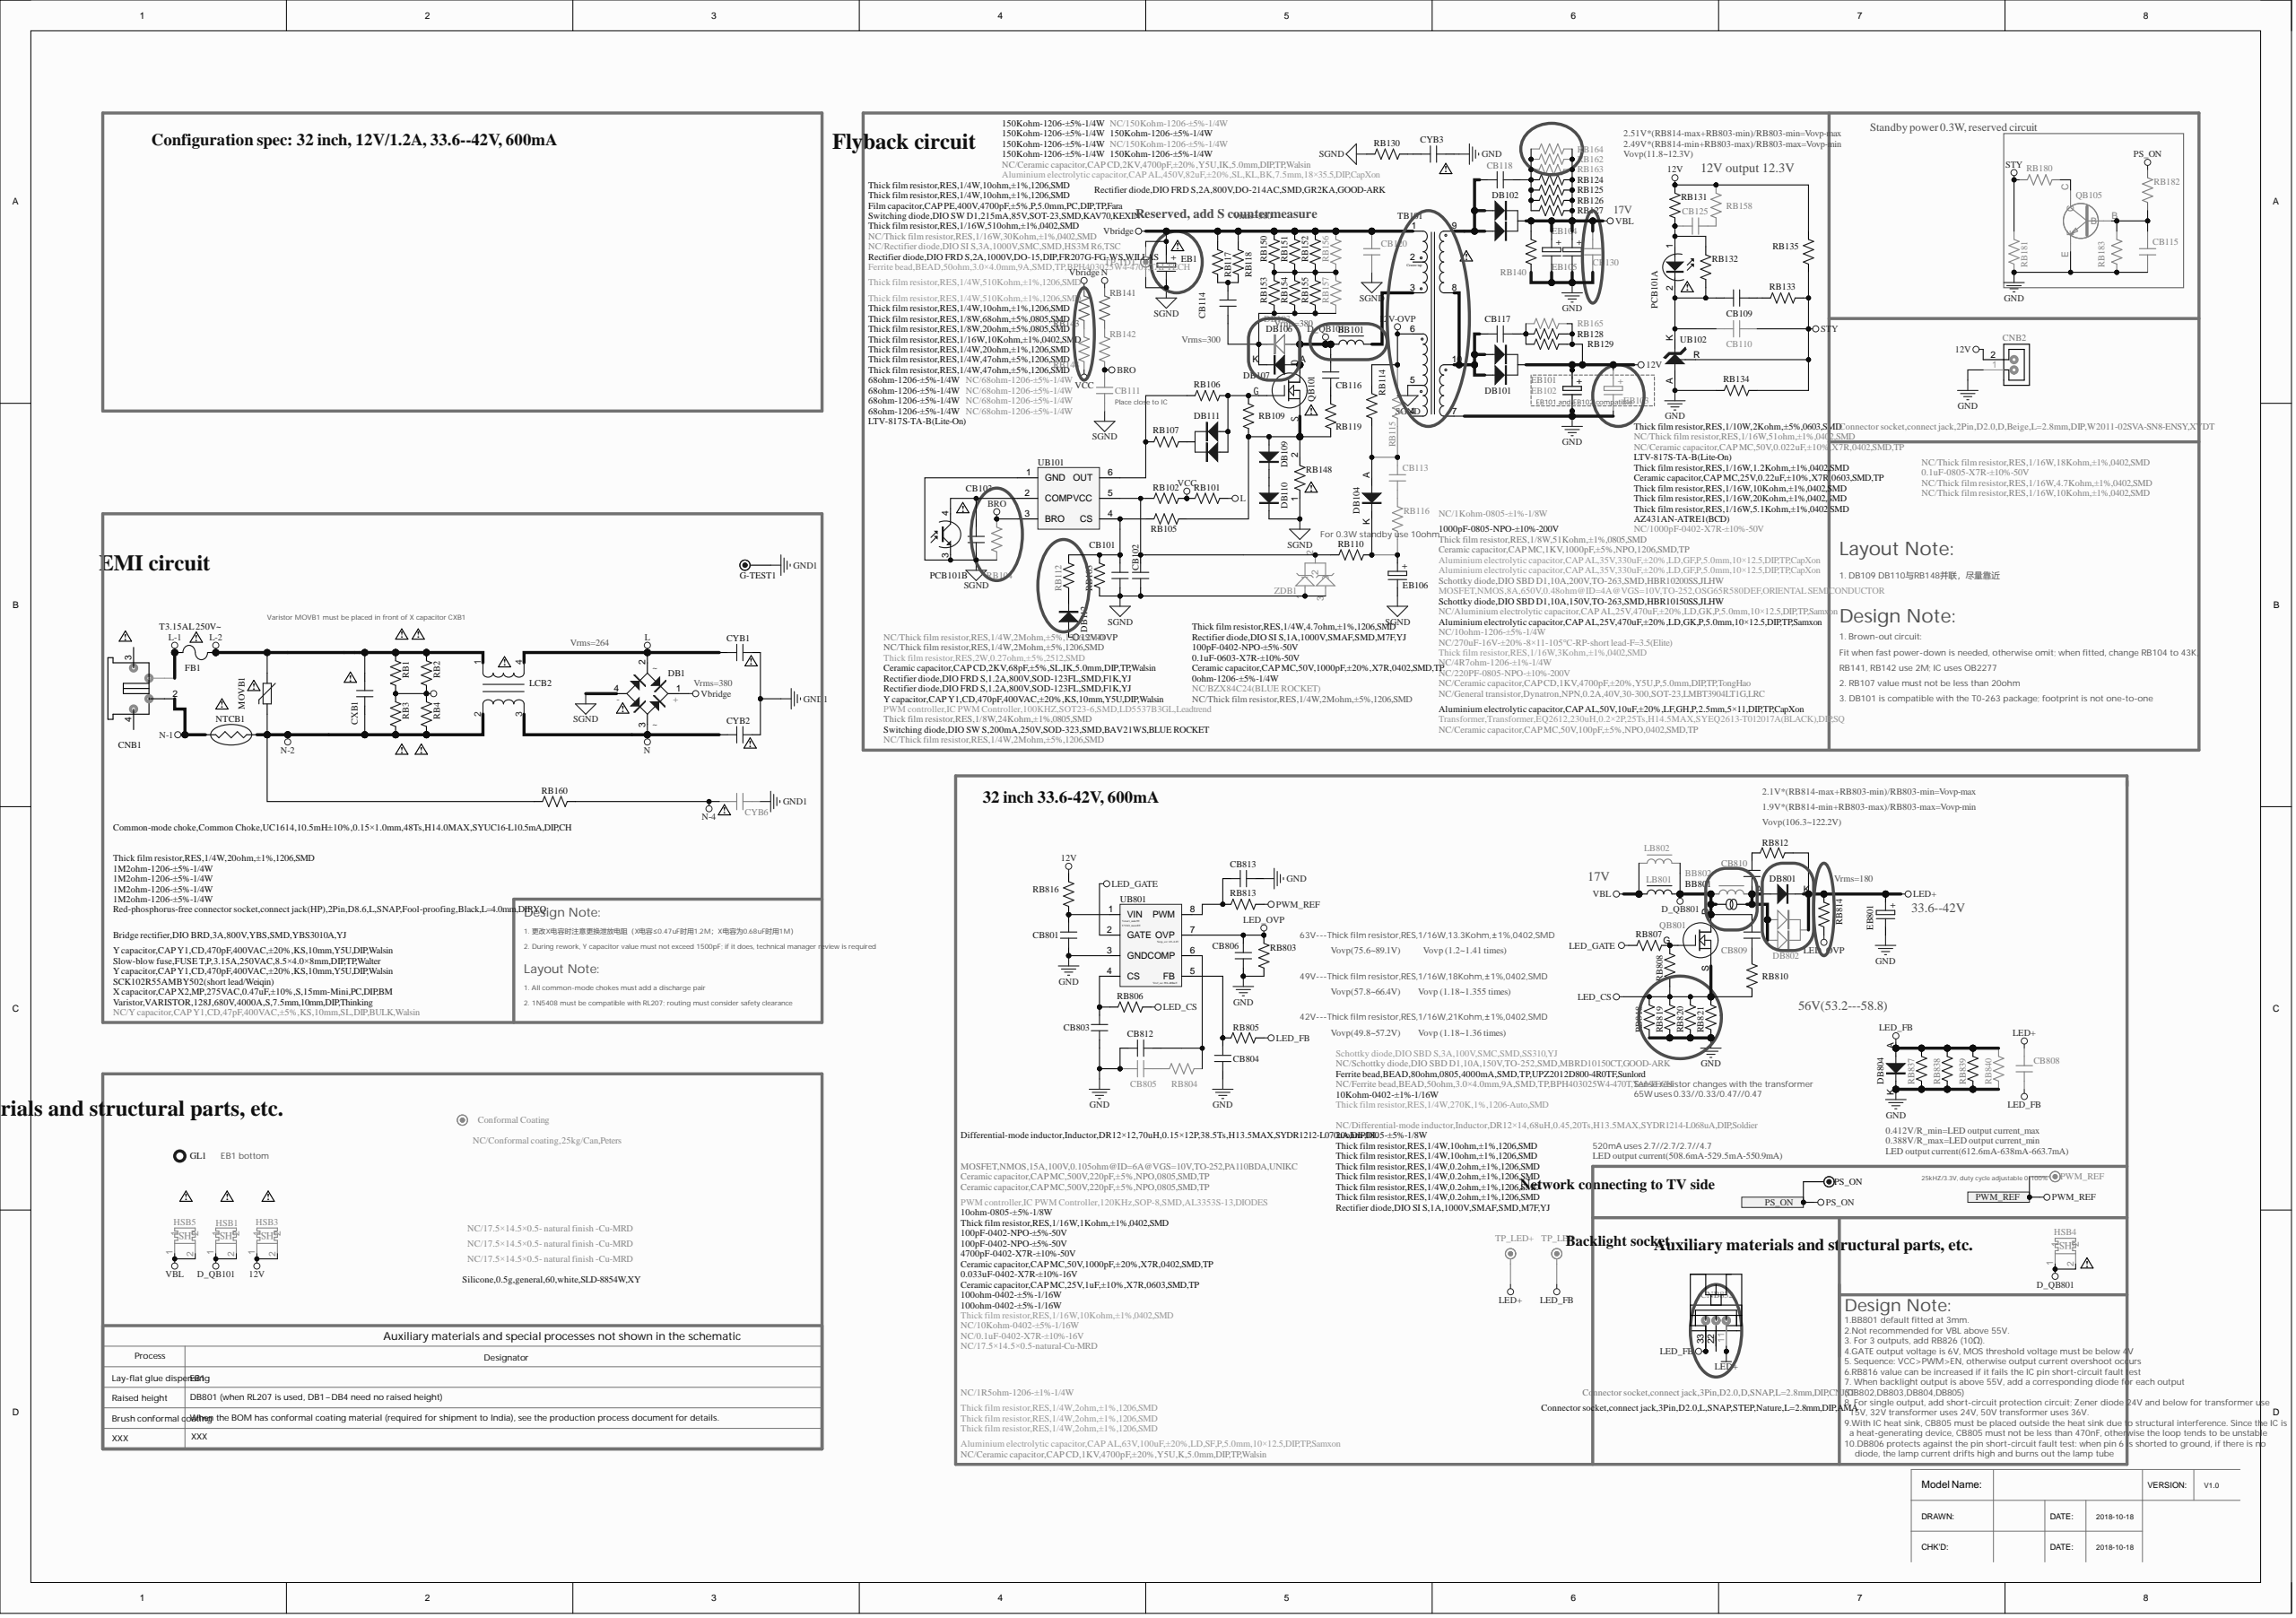Circuit board | Altium Designer | 719 parts | 352 nets | one sheet of the schematic
Parts on this sheet (reference | value | footprint):
BB101 | Ferrite bead,BEAD,50ohm,3.0×4.0mm,9A,SMD,TP,BPH403025W4-470T,TAI-TECH | L(4*3*2.55)-S
BB801 | Ferrite bead,BEAD,80ohm,0805,4000mA,SMD,TP,UPZ2012D800-4R0TF,Sunlord | R0805
BB802 | NC/Ferrite bead,BEAD,50ohm,3.0×4.0mm,9A,SMD,TP,BPH403025W4-470T,TAI-TECH | L(4*3*2.55)-S
CB101 | 100pF-0402-NPO-±5%-50V | C0402
CB102 | 0.1uF-0603-X7R-±10%-50V | C0603
CB103 | Ceramic capacitor,CAP MC,50V,1000pF,±20%,X7R,0402,SMD,TP | C0402
CB109 | Ceramic capacitor,CAP MC,25V,0.22uF,±10%,X7R,0603,SMD,TP | C0603
CB110 | NC/1000pF-0402-X7R-±10%-50V | C0402
CB111 | NC/Ceramic capacitor,CAP MC,50V,100pF,±5%,NPO,0402,SMD,TP | C0402
CB113 | NC/220PF-0805-NPO-±10%-200V | C0805
CB114 | Film capacitor,CAP PE,400V,4700pF,±5%,P,5.0mm,PC,DIP,TP,Fara | CAP8*2.5-V-5
CB115 | 0.1uF-0805-X7R-±10%-50V | C0805
CB116 | Ceramic capacitor,CAP CD,2KV,68pF,±5%,SL,IK,5.0mm,DIP,TP,Walsin | CAP6.5*5-V-5-1
CB117 | 1000pF-0805-NPO-±10%-200V | C0805
CB118 | Ceramic capacitor,CAP MC,1KV,1000pF,±5%,NPO,1206,SMD,TP | C1206
CB120 | NC/Ceramic capacitor,CAP CD,2KV,4700pF,±20%,Y5U,IK,5.0mm,DIP,TP,Walsin | CAP10*4.5-V-5
CB125 | NC/Ceramic capacitor,CAP MC,50V,0.022uF,±10%,X7R,0402,SMD,TP | C0402
CB130 | NC/Ceramic capacitor,CAP CD,1KV,4700pF,±20%,Y5U,P,5.0mm,DIP,TP,TongHao | CAP9.8*4-V-5
CB801 | Ceramic capacitor,CAP MC,25V,1uF,±10%,X7R,0603,SMD,TP | C0603
CB803 | 100pF-0402-NPO-±5%-50V | C0402
CB804 | 4700pF-0402-X7R-±10%-50V | C0402
CB805 | NC/0.1uF-0402-X7R-±10%-16V | C0402
CB806 | Ceramic capacitor,CAP MC,50V,1000pF,±20%,X7R,0402,SMD,TP | C0402
CB808 | NC/Ceramic capacitor,CAP CD,1KV,4700pF,±20%,Y5U,K,5.0mm,DIP,TP,Walsin | CAP10*4.5-V-5
CB809 | Ceramic capacitor,CAP MC,500V,220pF,±5%,NPO,0805,SMD,TP | C0805
CB810 | Ceramic capacitor,CAP MC,500V,220pF,±5%,NPO,0805,SMD,TP | C0805
CB812 | 0.033uF-0402-X7R-±10%-16V | C0402
CB813 | 100pF-0402-NPO-±5%-50V | C0402
CNB1 | Red-phosphorus-free connector socket,connect jack(HP),2Pin,D8.6,L,SNAP,Fool-proofing,Black,L=4.0mm,DIP,YQ | CON2-H8.6-1
CNB2 | Connector socket,connect jack,2Pin,D2.0,D,Beige,L=2.8mm,DIP,W2011-02SVA-SN8-ENSY,XYDT | SIP2/2.0D-1
CNB832 | Connector socket,connect jack,3Pin,D2.0,D,SNAP,L=2.8mm,DIP,CNJST | SIP3/2.0D-CP
CXB1 | X capacitor,CAP X2,MP,275VAC,0.47uF,±10%,S,15mm-Mini,PC,DIP,BM | CAP18*8.5-V-15
CYB1 | Y capacitor,CAP Y1,CD,470pF,400VAC,±20%,KS,10mm,Y5U,DIP,Walsin | CAP13*5-V-10-1
CYB2 | Y capacitor,CAP Y1,CD,470pF,400VAC,±20%,KS,10mm,Y5U,DIP,Walsin | CAP13*5-V-10-1
CYB3 | Y capacitor,CAP Y1,CD,470pF,400VAC,±20%,KS,10mm,Y5U,DIP,Walsin | CAP13*5-V-10-1
CYB6 | NC/Y capacitor,CAP Y1,CD,47pF,400VAC,±5%,KS,10mm,SL,DIP,BULK,Walsin | CAP13*5-V-10-1
DB1 | Bridge rectifier,DIO BRD,3A,800V,YBS,SMD,YBS3010A,YJ | B/YBS3010A
DB101 | Schottky diode,DIO SBD D1,10A,150V,TO-263,SMD,HBR10150SS,JLHW | D2PAK3
DB102 | Schottky diode,DIO SBD D1,10A,200V,TO-263,SMD,HBR10200SS,JLHW | D2PAK3
DB103 | NC/Rectifier diode,DIO SI S,3A,1000V,SMC,SMD,HS3M R6,TSC | DIODE-SMC
DB104 | Rectifier diode,DIO SI S,1A,1000V,SMAF,SMD,M7F,YJ | DIODE-S-2
DB106 | Rectifier diode,DIO FRD S,2A,1000V,DO-15,DIP,FR207G-FG-WS,WILLAS | D2-H-15
DB107 | Rectifier diode,DIO FRD S,2A,800V,DO-214AC,SMD,GR2KA,GOOD-ARK | DIODE-S-2
DB109 | Rectifier diode,DIO FRD S,1.2A,800V,SOD-123FL,SMD,F1K,YJ | DIODE-S-14
DB110 | Rectifier diode,DIO FRD S,1.2A,800V,SOD-123FL,SMD,F1K,YJ | DIODE-S-14
DB111 | Switching diode,DIO SW D1,215mA,85V,SOT-23,SMD,KAV70,KEXIN | SO-23
DB112 | Switching diode,DIO SW S,200mA,250V,SOD-323,SMD,BAV21WS,BLUE ROCKET | DIODE-S-12
DB801 | Schottky diode,DIO SBD S,3A,100V,SMC,SMD,SS310,YJ | DIODE-SMC
DB802 | NC/Schottky diode,DIO SBD D1,10A,150V,TO-252,SMD,MBRD10150CT,GOOD-ARK | TO-252
DB804 | Rectifier diode,DIO SI S,1A,1000V,SMAF,SMD,M7F,YJ | DIODE-S-2
EB1 | Aluminium electrolytic capacitor,CAP AL,450V,82uF,±20%,SL,KL,BK,7.5mm,18×35.5,DIP,CapXon | EC(18*36)-H7.5-1
EB101 | Aluminium electrolytic capacitor,CAP AL,25V,470uF,±20%,LD,GK,P,5.0mm,10×12.5,DIP,TP,Samxon | EC(10*12.5)-V-5
EB102 | NC/270uF-16V-±20%-8×11-105℃-RP-short lead-F=3.5(Elite) | EC(8*11)-V-3.5
EB103 | NC/Aluminium electrolytic capacitor,CAP AL,25V,470uF,±20%,LD,GK,P,5.0mm,10×12.5,DIP,TP,Samxon | EC(10*12.5)-V-5
EB105 | Aluminium electrolytic capacitor,CAP AL,35V,330uF,±20%,LD,GF,P,5.0mm,10×12.5,DIP,TP,CapXon | EC(10*12.5)-V-5
EB106 | Aluminium electrolytic capacitor,CAP AL,50V,10uF,±20%,LF,GH,P,2.5mm,5×11,DIP,TP,CapXon | EC(5*11)-V-2.5
EB801 | Aluminium electrolytic capacitor,CAP AL,63V,100uF,±20%,LD,SF,P,5.0mm,10×12.5,DIP,TP,Samxon | EC(10*12.5)-V-5
FB1 | Slow-blow fuse,FUSE T,P,3.15A,250VAC,8.5×4.0×8mm,DIP,TP,Walter | FUSE8.5*4-V-5(T3.15AL 250V~)
G-TEST1 | TEST | TP
GL1 | Silicone,0.5g,general,60,white,SLD-8854W,XY | Silica gel-20
HSB1 | NC/17.5×14.5×0.5- natural finish -Cu-MRD | HS038
HSB3 | NC/17.5×14.5×0.5- natural finish -Cu-MRD | HS038
HSB4 | NC/17.5×14.5×0.5-natural-Cu-MRD | HS038
HSB5 | NC/17.5×14.5×0.5- natural finish -Cu-MRD | HS038
LB801 | Differential-mode inductor,Inductor,DR12×12,70uH,0.15×12P,38.5Ts,H13.5MAX,SYDR1212-L070uA,DIP,DL | L/LC2/15*14.5-V7.5
LB802 | NC/Differential-mode inductor,Inductor,DR12×14,68uH,0.45,20Ts,H13.5MAX,SYDR1214-L068uA,DIP,Soldier | L(13.5*15.5)-V-5
LCB2 | Common-mode choke,Common Choke,UC1614,10.5mH±10%,0.15×1.0mm,48Ts,H14.0MAX,SYUC16-L10.5mA,DIP,CH | L/LC4/21*17-H-17*13
MOVB1 | Varistor,VARISTOR,128J,680V,4000A,S,7.5mm,10mm,DIP,Thinking | VR(13*5)-V-7.5
NTCB1 | SCK102R55AMBY502(short lead/Weiqin) | NTC(10*5)-V5
QB101 | MOSFET,NMOS,8A,650V,0.48ohm@ID=4A@VGS=10V,TO-252,OSG65R580DEF,ORIENTAL SEMICONDUCTOR | D2PAK3
QB105 | NC/General transistor,Dynatron,NPN,0.2A,40V,30-300,SOT-23,LMBT3904LT1G,LRC | SOT-23
QB801 | MOSFET,NMOS,15A,100V,0.105ohm@ID=6A@VGS=10V,TO-252,PA110BDA,UNIKC | TO-252-GDS
RB1 | 1M2ohm-1206-±5%-1/4W | R1206
RB2 | 1M2ohm-1206-±5%-1/4W | R1206
RB3 | 1M2ohm-1206-±5%-1/4W | R1206
RB4 | 1M2ohm-1206-±5%-1/4W | R1206
RB101 | Thick film resistor,RES,1/4W,510Kohm,±1%,1206,SMD | R1206
RB102 | Thick film resistor,RES,1/4W,510Kohm,±1%,1206,SMD | R1206
RB103 | Thick film resistor,RES,1/16W,3Kohm,±1%,0402,SMD | R0402
RB104 | NC/Thick film resistor,RES,1/16W,30Kohm,±1%,0402,SMD | R0402
RB105 | Thick film resistor,RES,1/16W,510ohm,±1%,0402,SMD | R0402
RB106 | Thick film resistor,RES,1/8W,68ohm,±5%,0805,SMD | R0805
RB107 | Thick film resistor,RES,1/8W,20ohm,±5%,0805,SMD | R0805
RB109 | Thick film resistor,RES,1/16W,10Kohm,±1%,0402,SMD | R0402
RB110 | 0ohm-1206-±5%-1/4W | R1206
RB112 | Thick film resistor,RES,1/8W,24Kohm,±1%,0805,SMD | R0805
RB114 | Thick film resistor,RES,1/4W,4.7ohm,±1%,1206,SMD | R1206
RB115 | NC/4R7ohm-1206-±1%-1/4W | R1206
RB116 | NC/10ohm-1206-±5%-1/4W | R1206
RB117 | Thick film resistor,RES,1/4W,10ohm,±1%,1206,SMD | R1206
RB118 | Thick film resistor,RES,1/4W,10ohm,±1%,1206,SMD | R1206
RB119 | Thick film resistor,RES,1/4W,10ohm,±1%,1206,SMD | R1206
RB124 | 68ohm-1206-±5%-1/4W | R1206
RB125 | 68ohm-1206-±5%-1/4W | R1206
RB126 | 68ohm-1206-±5%-1/4W | R1206
RB127 | 68ohm-1206-±5%-1/4W | R1206
RB128 | Thick film resistor,RES,1/4W,47ohm,±5%,1206,SMD | R1206
RB129 | Thick film resistor,RES,1/4W,47ohm,±5%,1206,SMD | R1206
RB130 | Thick film resistor,RES,1/4W,20ohm,±1%,1206,SMD | R1206
RB131 | Thick film resistor,RES,1/10W,2Kohm,±5%,0603,SMD | R0603
RB132 | Thick film resistor,RES,1/16W,1.2Kohm,±1%,0402,SMD | R0402
RB133 | Thick film resistor,RES,1/16W,10Kohm,±1%,0402,SMD | R0402
RB134 | Thick film resistor,RES,1/16W,5.1Kohm,±1%,0402,SMD | R0402
RB135 | Thick film resistor,RES,1/16W,20Kohm,±1%,0402,SMD | R0402
RB140 | Thick film resistor,RES,1/8W,51Kohm,±1%,0805,SMD | R0805
RB141 | NC/Thick film resistor,RES,1/4W,2Mohm,±5%,1206,SMD | R1206
RB142 | NC/Thick film resistor,RES,1/4W,2Mohm,±5%,1206,SMD | R1206
RB143 | NC/Thick film resistor,RES,1/4W,2Mohm,±5%,1206,SMD | R1206
RB144 | NC/Thick film resistor,RES,1/4W,2Mohm,±5%,1206,SMD | R1206
RB148 | Thick film resistor,RES,2W,0.27ohm,±5%,2512,SMD | R2512-1
RB150 | 150Kohm-1206-±5%-1/4W | R1206
RB151 | 150Kohm-1206-±5%-1/4W | R1206
RB152 | 150Kohm-1206-±5%-1/4W | R1206
RB153 | 150Kohm-1206-±5%-1/4W | R1206
RB154 | 150Kohm-1206-±5%-1/4W | R1206
RB155 | 150Kohm-1206-±5%-1/4W | R1206
RB156 | NC/150Kohm-1206-±5%-1/4W | R1206
RB157 | NC/150Kohm-1206-±5%-1/4W | R1206
RB158 | NC/Thick film resistor,RES,1/16W,51ohm,±1%,0402,SMD | R0402
RB160 | Thick film resistor,RES,1/4W,20ohm,±1%,1206,SMD | R1206
RB162 | NC/68ohm-1206-±5%-1/4W | R1206
RB163 | NC/68ohm-1206-±5%-1/4W | R1206
RB164 | NC/68ohm-1206-±5%-1/4W | R1206
RB165 | NC/68ohm-1206-±5%-1/4W | R1206
RB180 | NC/Thick film resistor,RES,1/16W,18Kohm,±1%,0402,SMD | R0402
RB181 | NC/1Kohm-0805-±1%-1/8W | R0805
RB182 | NC/Thick film resistor,RES,1/16W,4.7Kohm,±1%,0402,SMD | R0402
RB183 | NC/Thick film resistor,RES,1/16W,10Kohm,±1%,0402,SMD | R0402
RB803 | Thick film resistor,RES,1/16W,10Kohm,±1%,0402,SMD | R0402
RB804 | NC/10Kohm-0402-±5%-1/16W | R0402
RB805 | 100ohm-0402-±5%-1/16W | R0402
RB806 | Thick film resistor,RES,1/16W,1Kohm,±1%,0402,SMD | R0402
RB807 | 20ohm-0805-±5%-1/8W | R0805
RB808 | 10Kohm-0402-±1%-1/16W | R0402
RB810 | Thick film resistor,RES,1/4W,10ohm,±1%,1206,SMD | R1206
RB812 | Thick film resistor,RES,1/4W,10ohm,±1%,1206,SMD | R1206
RB813 | 100ohm-0402-±5%-1/16W | R0402
RB814 | Thick film resistor,RES,1/4W,270K,1%,1206-Auto,SMD | R1206
RB816 | 10ohm-0805-±5%-1/8W | R0805
RB818 | Thick film resistor,RES,1/4W,0.2ohm,±1%,1206,SMD | R1206
RB819 | Thick film resistor,RES,1/4W,0.2ohm,±1%,1206,SMD | R1206
RB820 | Thick film resistor,RES,1/4W,0.2ohm,±1%,1206,SMD | R1206
RB821 | Thick film resistor,RES,1/4W,0.2ohm,±1%,1206,SMD | R1206
RB837 | Thick film resistor,RES,1/4W,2ohm,±1%,1206,SMD | R1206
RB838 | Thick film resistor,RES,1/4W,2ohm,±1%,1206,SMD | R1206
RB839 | Thick film resistor,RES,1/4W,2ohm,±1%,1206,SMD | R1206
RB840 | NC/1R5ohm-1206-±1%-1/4W | R1206
TB101 | Transformer,Transformer,EQ2612,230uH,0.2×2P,25Ts,H14.5MAX,SYEQ2613-T012017A(BLACK),DIP,SQ | T/EQ2612*10
TP-TDT | NC/ | TP-TDT
TP_LED+ | NC/ | TP
UB101 | PWM controller,IC PWM Controller,100KHZ,SOT23-6,SMD,LD5537B3GL,Leadtrend | SOT-26
UB102 | AZ431AN-ATRE1(BCD) | SOT-23-RAK
UB801 | PWM controller,IC PWM Controller,120KHz,SOP-8,SMD,AL3353S-13,DIODES | SO-8A
ZDB1 | NC/BZX84C24(BLUE ROCKET) | SO-23
Nets of these parts (net: part-pin ...):
VCC: RB101-2 RB102-1 RB144-1
Vbridge: CB120-2 DB1-1 EB1-1 RB117-2 RB118-2 RB143-2 RB150-2 RB151-2 RB152-2 RB156-2 TB101-1 TP-TDT-1
VBL: CB130-2 DB102-2 EB105-1 HSB5-1 HSB5-2 LB801-1 LB802-1 RB124-2 RB125-2 RB126-2 RB127-2 RB140-1 RB162-2 RB163-2 RB164-2
STY: CB110-2 RB133-1 RB134-2 RB135-2 RB180-2 RB181-2 UB102-R
SGND: CB101-2 CB102-2 CB103-2 CB111-2 CB120-1 DB1-4 DB110-K EB1-2 EB106-2 RB103-1 RB104-1 RB130-1 RB148-1 TB101-5 TP-TDT-2 UB101-1 ZDB1-1 ZDB1-3
PWM_REF: RB813-2
PS_ON: RB182-2
NetRB150_1: RB150-1 RB151-1 RB152-1 RB153-2 RB154-2 RB155-2 RB156-1 RB157-2
NetRB143_1: RB143-1 RB144-2
NetRB141_1: RB141-1 RB142-2
NetRB106_1: RB106-1 RB107-1 UB101-6
NetQB801_G: QB801-G RB807-2 RB808-2
NetQB105_C: QB105-C RB180-1
NetDB112_K: DB112-K RB112-2
NetDB111_2: DB111-2 RB107-2
NetDB111_1: DB111-1 DB111-3 QB101-1 RB106-2 RB109-2
NetDB109_K: DB109-K DB110-A
NetDB109_A: DB109-A QB101-3 RB105-2 RB109-1 RB119-1 RB148-2
NetDB104_K: DB104-K EB106-1 RB110-2 RB116-2
NetCYB3_1: CYB3-1 RB130-2
NetCB813_2: CB813-2 RB813-1 UB801-8
NetCB812_2: CB812-2 RB804-2 UB801-6
NetCB810_2: CB810-2 RB812-1
NetCB809_1: CB809-1 RB810-1
NetCB805_2: CB805-2 RB804-1
NetCB804_1: CB804-1 RB805-1 UB801-5
NetCB803_1: CB803-1 RB806-1 UB801-4
NetCB801_2: CB801-2 RB816-2 UB801-1
NetCB125_2: CB125-2 RB158-1
NetCB125_1: CB125-1 RB131-1 RB132-2
NetCB118_2: CB118-2 RB124-1 RB125-1 RB126-1 RB127-1 RB162-1 RB163-1 RB164-1
NetCB118_1: CB118-1 DB102-1 DB102-3 TB101-9
NetCB117_2: CB117-2 RB128-1 RB129-1 RB165-1
NetCB117_1: CB117-1 DB101-1 DB101-3 TB101-8 TB101-10
NetCB116_1: CB116-1 RB119-2
NetCB115_1: CB115-1 QB105-B RB182-1 RB183-1
NetCB114_2: CB114-2 DB103-K DB106-K DB107-K RB153-1 RB154-1 RB155-1 RB157-1
NetCB114_1: CB114-1 RB117-1 RB118-1
NetCB113_2: CB113-2 RB116-1
NetCB113_1: CB113-1 DB104-A RB114-1 RB115-1
NetCB109_2: CB109-2 RB133-2
NetCB109_1: CB109-1 CB110-1 RB132-1 UB102-K
NetCB103_1: CB103-1 UB101-2
NetCB102_1: CB102-1 RB102-2 RB110-1 UB101-5 ZDB1-2
NetCB101_1: CB101-1 RB103-2 RB105-1 RB112-1 UB101-4
NetBB801_2: BB801-2 BB802-2 CB810-1 DB801-A DB802-1 DB802-3
NetBB101_2: BB101-2 TB101-3
N-4: CYB6-1 RB160-2
N-2: CXB1-2 LCB2-2 MOVB1-2 NTCB1-1 RB3-2 RB4-2 RB160-1
N-1: CNB1-2 NTCB1-2
N: CYB2-1 DB1-3 LCB2-3 RB141-2
LED_OVP: CB806-1 RB803-2 RB814-2 UB801-7
LED_GATE: RB807-1 UB801-2
LED_FB: CB808-1 CNB832-3 DB804-A RB805-2 RB837-2 RB838-2 RB839-1 RB840-2
LED_CS: QB801-S RB806-2 RB808-1 RB810-2 RB818-1 RB819-1 RB820-1 RB821-1
LED+: CB808-2 CNB832-1 DB801-K DB802-2 EB801-1 RB812-2 RB814-1 TP_LED+-1
L-N: RB1-2 RB2-2 RB3-1 RB4-1
L-2: CXB1-1 FB1-2 LCB2-1 MOVB1-1 RB1-1 RB2-1
L-1: CNB1-1 FB1-1
L: CYB1-1 DB1-2 LCB2-4 RB101-1
GND1: CYB1-2 CYB2-2 CYB6-2 G-TEST1-1
GND: CB115-2 CB130-1 CB801-1 CB803-2 CB804-2 CB805-1 CB806-2 CB812-1 CB813-1 CNB2-1 CYB3-2 DB804-K EB101-2 EB102-2 EB103-2 EB105-2 EB801-2 QB105-E RB134-1 RB140-2 RB181-1 RB183-2 RB803-1 RB818-2 RB819-2 RB820-2 RB821-2 RB837-1 RB838-1 RB839-2 RB840-1 TB101-7 UB102-A UB801-3
D_QB801: BB801-1 BB802-1 CB809-2 HSB4-1 HSB4-2 LB801-2 LB802-2 QB801-D
D_QB101: BB101-1 CB116-2 DB103-A DB106-A DB107-A HSB1-1 HSB1-2 QB101-2
BRO: CB111-1 RB104-2 RB142-1 UB101-3
12V-OVP: DB112-A RB114-2 RB115-2 TB101-6
12V: CNB2-2 DB101-2 EB101-1 EB102-1 EB103-1 HSB3-1 HSB3-2 RB128-2 RB129-2 RB131-2 RB135-1 RB158-2 RB165-2 RB816-1